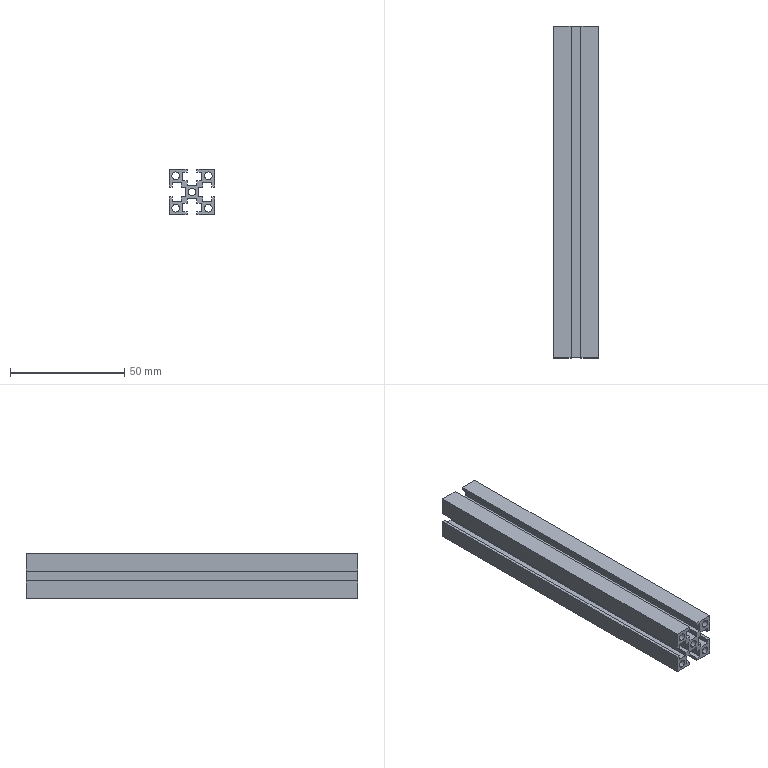Part | STEP file | 20 aluminium profile vertical 2 | 1 solid | 64 faces | box 20 x 145 x 20 mm | volume 25778 mm3 | plane 54 | cylinder 10 | commonest cylinder face diameters 3.3 x10